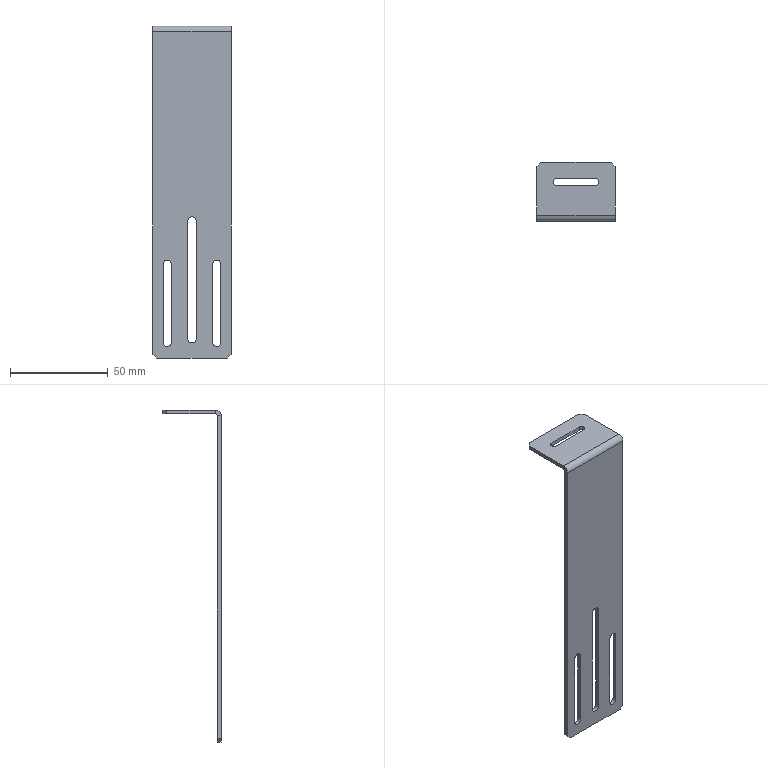Part | NX | 1 solid | 34 faces | box 40 x 30 x 170 mm | volume 14302 mm3 | plane 24 | cylinder 10 | commonest cylinder face diameters 4.2 x4 3.4 x2 4.5 x2 2 x1 6 x1
STEP:
#1=CARTESIAN_POINT('',(14.8,-2.,48.));
#2=VERTEX_POINT('',#1);
#3=CARTESIAN_POINT('',(14.8,-2.,8.));
#4=VERTEX_POINT('',#3);
#5=CARTESIAN_POINT('',(14.8,-2.,8.));
#6=DIRECTION('',(0.,0.,-1.));
#7=VECTOR('',#6,1000.);
#8=LINE('',#5,#7);
#9=EDGE_CURVE('',#2,#4,#8,.T.);
#10=ORIENTED_EDGE('',*,*,#9,.T.);
#11=CARTESIAN_POINT('',(10.6,-2.,8.));
#12=VERTEX_POINT('',#11);
#13=CARTESIAN_POINT('',(12.7,-2.,8.));
#14=DIRECTION('',(0.,1.,0.));
#15=DIRECTION('',(-1.,0.,0.));
#16=AXIS2_PLACEMENT_3D('',#13,#14,#15);
#17=CIRCLE('',#16,2.1);
#18=EDGE_CURVE('',#4,#12,#17,.T.);
#19=ORIENTED_EDGE('',*,*,#18,.T.);
#20=CARTESIAN_POINT('',(10.6,-2.,48.));
#21=VERTEX_POINT('',#20);
#22=CARTESIAN_POINT('',(10.6,-2.,8.));
#23=DIRECTION('',(0.,0.,1.));
#24=VECTOR('',#23,1000.);
#25=LINE('',#22,#24);
#26=EDGE_CURVE('',#12,#21,#25,.T.);
#27=ORIENTED_EDGE('',*,*,#26,.T.);
#28=CARTESIAN_POINT('',(12.7,-2.,48.));
#29=DIRECTION('',(0.,1.,0.));
#30=DIRECTION('',(-1.,0.,0.));
#31=AXIS2_PLACEMENT_3D('',#28,#29,#30);
#32=CIRCLE('',#31,2.1);
#33=EDGE_CURVE('',#21,#2,#32,.T.);
#34=ORIENTED_EDGE('',*,*,#33,.T.);
#35=EDGE_LOOP('',(#10,#19,#27,#34));
#36=FACE_BOUND('',#35,.T.);
#37=CARTESIAN_POINT('',(-10.6,-2.,48.));
#38=VERTEX_POINT('',#37);
#39=CARTESIAN_POINT('',(-10.6,-2.,8.));
#40=VERTEX_POINT('',#39);
#41=CARTESIAN_POINT('',(-10.6,-2.,8.));
#42=DIRECTION('',(0.,0.,-1.));
#43=VECTOR('',#42,1000.);
#44=LINE('',#41,#43);
#45=EDGE_CURVE('',#38,#40,#44,.T.);
#46=ORIENTED_EDGE('',*,*,#45,.T.);
#47=CARTESIAN_POINT('',(-14.8,-2.,8.));
#48=VERTEX_POINT('',#47);
#49=CARTESIAN_POINT('',(-12.7,-2.,8.));
#50=DIRECTION('',(0.,1.,0.));
#51=DIRECTION('',(-1.,0.,0.));
#52=AXIS2_PLACEMENT_3D('',#49,#50,#51);
#53=CIRCLE('',#52,2.1);
#54=EDGE_CURVE('',#40,#48,#53,.T.);
#55=ORIENTED_EDGE('',*,*,#54,.T.);
#56=CARTESIAN_POINT('',(-14.8,-2.,48.));
#57=VERTEX_POINT('',#56);
#58=CARTESIAN_POINT('',(-14.8,-2.,8.));
#59=DIRECTION('',(0.,0.,1.));
#60=VECTOR('',#59,1000.);
#61=LINE('',#58,#60);
#62=EDGE_CURVE('',#48,#57,#61,.T.);
#63=ORIENTED_EDGE('',*,*,#62,.T.);
#64=CARTESIAN_POINT('',(-12.7,-2.,48.));
#65=DIRECTION('',(0.,1.,0.));
#66=DIRECTION('',(-1.,0.,0.));
#67=AXIS2_PLACEMENT_3D('',#64,#65,#66);
#68=CIRCLE('',#67,2.1);
#69=EDGE_CURVE('',#57,#38,#68,.T.);
#70=ORIENTED_EDGE('',*,*,#69,.T.);
#71=EDGE_LOOP('',(#46,#55,#63,#70));
#72=FACE_BOUND('',#71,.T.);
#73=CARTESIAN_POINT('',(2.25,-2.,10.));
#74=VERTEX_POINT('',#73);
#75=CARTESIAN_POINT('',(2.25,-2.,70.));
#76=VERTEX_POINT('',#75);
#77=CARTESIAN_POINT('',(2.25,-2.,10.));
#78=DIRECTION('',(0.,0.,1.));
#79=VECTOR('',#78,1000.);
#80=LINE('',#77,#79);
#81=EDGE_CURVE('',#74,#76,#80,.T.);
#82=ORIENTED_EDGE('',*,*,#81,.F.);
#83=CARTESIAN_POINT('',(-2.25,-2.,10.));
#84=VERTEX_POINT('',#83);
#85=CARTESIAN_POINT('',(0.,-2.,10.));
#86=DIRECTION('',(0.,-1.,0.));
#87=DIRECTION('',(0.,0.,-1.));
#88=AXIS2_PLACEMENT_3D('',#85,#86,#87);
#89=CIRCLE('',#88,2.25);
#90=EDGE_CURVE('',#84,#74,#89,.T.);
#91=ORIENTED_EDGE('',*,*,#90,.F.);
#92=CARTESIAN_POINT('',(-2.25,-2.,70.));
#93=VERTEX_POINT('',#92);
#94=CARTESIAN_POINT('',(-2.25,-2.,10.));
#95=DIRECTION('',(0.,0.,-1.));
#96=VECTOR('',#95,1000.);
#97=LINE('',#94,#96);
#98=EDGE_CURVE('',#93,#84,#97,.T.);
#99=ORIENTED_EDGE('',*,*,#98,.F.);
#100=CARTESIAN_POINT('',(0.,-2.,70.));
#101=DIRECTION('',(0.,-1.,0.));
#102=DIRECTION('',(0.,0.,-1.));
#103=AXIS2_PLACEMENT_3D('',#100,#101,#102);
#104=CIRCLE('',#103,2.25);
#105=EDGE_CURVE('',#76,#93,#104,.T.);
#106=ORIENTED_EDGE('',*,*,#105,.F.);
#107=EDGE_LOOP('',(#82,#91,#99,#106));
#108=FACE_BOUND('',#107,.T.);
#109=CARTESIAN_POINT('',(-20.,-2.,167.));
#110=VERTEX_POINT('',#109);
#111=CARTESIAN_POINT('',(-20.,-2.,2.));
#112=VERTEX_POINT('',#111);
#113=CARTESIAN_POINT('',(-20.,-2.,170.));
#114=DIRECTION('',(0.,0.,-1.));
#115=VECTOR('',#114,1000.);
#116=LINE('',#113,#115);
#117=EDGE_CURVE('',#110,#112,#116,.T.);
#118=ORIENTED_EDGE('',*,*,#117,.T.);
#119=CARTESIAN_POINT('',(-18.,-2.,0.));
#120=VERTEX_POINT('',#119);
#121=CARTESIAN_POINT('',(-18.,-2.,0.));
#122=DIRECTION('',(-0.7071,0.,0.7071));
#123=VECTOR('',#122,1000.);
#124=LINE('',#121,#123);
#125=EDGE_CURVE('',#112,#120,#124,.F.);
#126=ORIENTED_EDGE('',*,*,#125,.T.);
#127=CARTESIAN_POINT('',(18.,-2.,0.));
#128=VERTEX_POINT('',#127);
#129=CARTESIAN_POINT('',(-20.,-2.,0.));
#130=DIRECTION('',(1.,0.,0.));
#131=VECTOR('',#130,1000.);
#132=LINE('',#129,#131);
#133=EDGE_CURVE('',#120,#128,#132,.T.);
#134=ORIENTED_EDGE('',*,*,#133,.T.);
#135=CARTESIAN_POINT('',(20.,-2.,2.));
#136=VERTEX_POINT('',#135);
#137=CARTESIAN_POINT('',(18.,-2.,0.));
#138=DIRECTION('',(-0.7071,0.,-0.7071));
#139=VECTOR('',#138,1000.);
#140=LINE('',#137,#139);
#141=EDGE_CURVE('',#128,#136,#140,.F.);
#142=ORIENTED_EDGE('',*,*,#141,.T.);
#143=CARTESIAN_POINT('',(20.,-2.,167.));
#144=VERTEX_POINT('',#143);
#145=CARTESIAN_POINT('',(20.,-2.,170.));
#146=DIRECTION('',(0.,0.,-1.));
#147=VECTOR('',#146,1000.);
#148=LINE('',#145,#147);
#149=EDGE_CURVE('',#144,#136,#148,.T.);
#150=ORIENTED_EDGE('',*,*,#149,.F.);
#151=CARTESIAN_POINT('',(20.,-2.,167.));
#152=DIRECTION('',(1.,0.,0.));
#153=VECTOR('',#152,1000.);
#154=LINE('',#151,#153);
#155=EDGE_CURVE('',#144,#110,#154,.F.);
#156=ORIENTED_EDGE('',*,*,#155,.T.);
#157=EDGE_LOOP('',(#118,#126,#134,#142,#150,#156));
#158=FACE_BOUND('',#157,.T.);
#159=CARTESIAN_POINT('',(-20.,-2.,170.));
#160=DIRECTION('',(0.,1.,0.));
#161=DIRECTION('',(0.,0.,1.));
#162=AXIS2_PLACEMENT_3D('',#159,#160,#161);
#163=PLANE('',#162);
#164=ADVANCED_FACE('',(#36,#72,#108,#158),#163,.F.);
#165=ORIENTED_EDGE('',*,*,#149,.T.);
#166=CARTESIAN_POINT('',(20.,0.,2.));
#167=VERTEX_POINT('',#166);
#168=CARTESIAN_POINT('',(20.,0.,2.));
#169=DIRECTION('',(0.,1.,0.));
#170=VECTOR('',#169,1000.);
#171=LINE('',#168,#170);
#172=EDGE_CURVE('',#136,#167,#171,.T.);
#173=ORIENTED_EDGE('',*,*,#172,.T.);
#174=CARTESIAN_POINT('',(20.,0.,167.));
#175=VERTEX_POINT('',#174);
#176=CARTESIAN_POINT('',(20.,0.,170.));
#177=DIRECTION('',(0.,0.,-1.));
#178=VECTOR('',#177,1000.);
#179=LINE('',#176,#178);
#180=EDGE_CURVE('',#175,#167,#179,.T.);
#181=ORIENTED_EDGE('',*,*,#180,.F.);
#182=CARTESIAN_POINT('',(20.,0.,167.));
#183=DIRECTION('',(0.,-1.,0.));
#184=VECTOR('',#183,1000.);
#185=LINE('',#182,#184);
#186=EDGE_CURVE('',#175,#144,#185,.T.);
#187=ORIENTED_EDGE('',*,*,#186,.T.);
#188=EDGE_LOOP('',(#165,#173,#181,#187));
#189=FACE_BOUND('',#188,.T.);
#190=CARTESIAN_POINT('',(20.,0.,170.));
#191=DIRECTION('',(1.,0.,0.));
#192=DIRECTION('',(0.,0.,-1.));
#193=AXIS2_PLACEMENT_3D('',#190,#191,#192);
#194=PLANE('',#193);
#195=ADVANCED_FACE('',(#189),#194,.T.);
#196=CARTESIAN_POINT('',(14.8,0.,8.));
#197=VERTEX_POINT('',#196);
#198=CARTESIAN_POINT('',(10.6,0.,8.));
#199=VERTEX_POINT('',#198);
#200=CARTESIAN_POINT('',(12.7,0.,8.));
#201=DIRECTION('',(0.,1.,0.));
#202=DIRECTION('',(-1.,0.,0.));
#203=AXIS2_PLACEMENT_3D('',#200,#201,#202);
#204=CIRCLE('',#203,2.1);
#205=EDGE_CURVE('',#197,#199,#204,.T.);
#206=ORIENTED_EDGE('',*,*,#205,.F.);
#207=CARTESIAN_POINT('',(14.8,0.,48.));
#208=VERTEX_POINT('',#207);
#209=CARTESIAN_POINT('',(14.8,0.,8.));
#210=DIRECTION('',(0.,0.,-1.));
#211=VECTOR('',#210,1000.);
#212=LINE('',#209,#211);
#213=EDGE_CURVE('',#208,#197,#212,.T.);
#214=ORIENTED_EDGE('',*,*,#213,.F.);
#215=CARTESIAN_POINT('',(10.6,0.,48.));
#216=VERTEX_POINT('',#215);
#217=CARTESIAN_POINT('',(12.7,0.,48.));
#218=DIRECTION('',(0.,1.,0.));
#219=DIRECTION('',(-1.,0.,0.));
#220=AXIS2_PLACEMENT_3D('',#217,#218,#219);
#221=CIRCLE('',#220,2.1);
#222=EDGE_CURVE('',#216,#208,#221,.T.);
#223=ORIENTED_EDGE('',*,*,#222,.F.);
#224=CARTESIAN_POINT('',(10.6,0.,8.));
#225=DIRECTION('',(0.,0.,1.));
#226=VECTOR('',#225,1000.);
#227=LINE('',#224,#226);
#228=EDGE_CURVE('',#199,#216,#227,.T.);
#229=ORIENTED_EDGE('',*,*,#228,.F.);
#230=EDGE_LOOP('',(#206,#214,#223,#229));
#231=FACE_BOUND('',#230,.T.);
#232=CARTESIAN_POINT('',(-10.6,0.,8.));
#233=VERTEX_POINT('',#232);
#234=CARTESIAN_POINT('',(-14.8,0.,8.));
#235=VERTEX_POINT('',#234);
#236=CARTESIAN_POINT('',(-12.7,0.,8.));
#237=DIRECTION('',(0.,1.,0.));
#238=DIRECTION('',(-1.,0.,0.));
#239=AXIS2_PLACEMENT_3D('',#236,#237,#238);
#240=CIRCLE('',#239,2.1);
#241=EDGE_CURVE('',#233,#235,#240,.T.);
#242=ORIENTED_EDGE('',*,*,#241,.F.);
#243=CARTESIAN_POINT('',(-10.6,0.,48.));
#244=VERTEX_POINT('',#243);
#245=CARTESIAN_POINT('',(-10.6,0.,8.));
#246=DIRECTION('',(0.,0.,-1.));
#247=VECTOR('',#246,1000.);
#248=LINE('',#245,#247);
#249=EDGE_CURVE('',#244,#233,#248,.T.);
#250=ORIENTED_EDGE('',*,*,#249,.F.);
#251=CARTESIAN_POINT('',(-14.8,0.,48.));
#252=VERTEX_POINT('',#251);
#253=CARTESIAN_POINT('',(-12.7,0.,48.));
#254=DIRECTION('',(0.,1.,0.));
#255=DIRECTION('',(-1.,0.,0.));
#256=AXIS2_PLACEMENT_3D('',#253,#254,#255);
#257=CIRCLE('',#256,2.1);
#258=EDGE_CURVE('',#252,#244,#257,.T.);
#259=ORIENTED_EDGE('',*,*,#258,.F.);
#260=CARTESIAN_POINT('',(-14.8,0.,8.));
#261=DIRECTION('',(0.,0.,1.));
#262=VECTOR('',#261,1000.);
#263=LINE('',#260,#262);
#264=EDGE_CURVE('',#235,#252,#263,.T.);
#265=ORIENTED_EDGE('',*,*,#264,.F.);
#266=EDGE_LOOP('',(#242,#250,#259,#265));
#267=FACE_BOUND('',#266,.T.);
#268=CARTESIAN_POINT('',(-2.25,0.,10.));
#269=VERTEX_POINT('',#268);
#270=CARTESIAN_POINT('',(2.25,0.,10.));
#271=VERTEX_POINT('',#270);
#272=CARTESIAN_POINT('',(0.,0.,10.));
#273=DIRECTION('',(0.,-1.,0.));
#274=DIRECTION('',(0.,0.,-1.));
#275=AXIS2_PLACEMENT_3D('',#272,#273,#274);
#276=CIRCLE('',#275,2.25);
#277=EDGE_CURVE('',#269,#271,#276,.T.);
#278=ORIENTED_EDGE('',*,*,#277,.T.);
#279=CARTESIAN_POINT('',(2.25,0.,70.));
#280=VERTEX_POINT('',#279);
#281=CARTESIAN_POINT('',(2.25,0.,10.));
#282=DIRECTION('',(0.,0.,1.));
#283=VECTOR('',#282,1000.);
#284=LINE('',#281,#283);
#285=EDGE_CURVE('',#271,#280,#284,.T.);
#286=ORIENTED_EDGE('',*,*,#285,.T.);
#287=CARTESIAN_POINT('',(-2.25,0.,70.));
#288=VERTEX_POINT('',#287);
#289=CARTESIAN_POINT('',(0.,0.,70.));
#290=DIRECTION('',(0.,-1.,0.));
#291=DIRECTION('',(0.,0.,-1.));
#292=AXIS2_PLACEMENT_3D('',#289,#290,#291);
#293=CIRCLE('',#292,2.25);
#294=EDGE_CURVE('',#280,#288,#293,.T.);
#295=ORIENTED_EDGE('',*,*,#294,.T.);
#296=CARTESIAN_POINT('',(-2.25,0.,10.));
#297=DIRECTION('',(0.,0.,-1.));
#298=VECTOR('',#297,1000.);
#299=LINE('',#296,#298);
#300=EDGE_CURVE('',#288,#269,#299,.T.);
#301=ORIENTED_EDGE('',*,*,#300,.T.);
#302=EDGE_LOOP('',(#278,#286,#295,#301));
#303=FACE_BOUND('',#302,.T.);
#304=CARTESIAN_POINT('',(-18.,0.,0.));
#305=VERTEX_POINT('',#304);
#306=CARTESIAN_POINT('',(18.,0.,0.));
#307=VERTEX_POINT('',#306);
#308=CARTESIAN_POINT('',(-20.,0.,0.));
#309=DIRECTION('',(1.,0.,0.));
#310=VECTOR('',#309,1000.);
#311=LINE('',#308,#310);
#312=EDGE_CURVE('',#305,#307,#311,.T.);
#313=ORIENTED_EDGE('',*,*,#312,.F.);
#314=CARTESIAN_POINT('',(-20.,0.,2.));
#315=VERTEX_POINT('',#314);
#316=CARTESIAN_POINT('',(-104.,0.,86.));
#317=DIRECTION('',(0.7071,0.,-0.7071));
#318=VECTOR('',#317,1000.);
#319=LINE('',#316,#318);
#320=EDGE_CURVE('',#305,#315,#319,.F.);
#321=ORIENTED_EDGE('',*,*,#320,.T.);
#322=CARTESIAN_POINT('',(-20.,0.,167.));
#323=VERTEX_POINT('',#322);
#324=CARTESIAN_POINT('',(-20.,0.,170.));
#325=DIRECTION('',(0.,0.,-1.));
#326=VECTOR('',#325,1000.);
#327=LINE('',#324,#326);
#328=EDGE_CURVE('',#323,#315,#327,.T.);
#329=ORIENTED_EDGE('',*,*,#328,.F.);
#330=CARTESIAN_POINT('',(20.,0.,167.));
#331=DIRECTION('',(1.,0.,0.));
#332=VECTOR('',#331,1000.);
#333=LINE('',#330,#332);
#334=EDGE_CURVE('',#175,#323,#333,.F.);
#335=ORIENTED_EDGE('',*,*,#334,.F.);
#336=ORIENTED_EDGE('',*,*,#180,.T.);
#337=CARTESIAN_POINT('',(84.,0.,66.));
#338=DIRECTION('',(0.7071,0.,0.7071));
#339=VECTOR('',#338,1000.);
#340=LINE('',#337,#339);
#341=EDGE_CURVE('',#167,#307,#340,.F.);
#342=ORIENTED_EDGE('',*,*,#341,.T.);
#343=EDGE_LOOP('',(#313,#321,#329,#335,#336,#342));
#344=FACE_BOUND('',#343,.T.);
#345=CARTESIAN_POINT('',(-20.,0.,170.));
#346=DIRECTION('',(0.,1.,0.));
#347=DIRECTION('',(0.,0.,1.));
#348=AXIS2_PLACEMENT_3D('',#345,#346,#347);
#349=PLANE('',#348);
#350=ADVANCED_FACE('',(#231,#267,#303,#344),#349,.T.);
#351=ORIENTED_EDGE('',*,*,#328,.T.);
#352=CARTESIAN_POINT('',(-20.,-2.,2.));
#353=DIRECTION('',(0.,-1.,0.));
#354=VECTOR('',#353,1000.);
#355=LINE('',#352,#354);
#356=EDGE_CURVE('',#315,#112,#355,.T.);
#357=ORIENTED_EDGE('',*,*,#356,.T.);
#358=ORIENTED_EDGE('',*,*,#117,.F.);
#359=CARTESIAN_POINT('',(-20.,0.,167.));
#360=DIRECTION('',(0.,-1.,0.));
#361=VECTOR('',#360,1000.);
#362=LINE('',#359,#361);
#363=EDGE_CURVE('',#323,#110,#362,.T.);
#364=ORIENTED_EDGE('',*,*,#363,.F.);
#365=EDGE_LOOP('',(#351,#357,#358,#364));
#366=FACE_BOUND('',#365,.T.);
#367=CARTESIAN_POINT('',(-20.,-2.,170.));
#368=DIRECTION('',(-1.,0.,0.));
#369=DIRECTION('',(0.,0.,1.));
#370=AXIS2_PLACEMENT_3D('',#367,#368,#369);
#371=PLANE('',#370);
#372=ADVANCED_FACE('',(#366),#371,.T.);
#373=ORIENTED_EDGE('',*,*,#133,.F.);
#374=CARTESIAN_POINT('',(-18.,0.,0.));
#375=DIRECTION('',(0.,1.,0.));
#376=VECTOR('',#375,1000.);
#377=LINE('',#374,#376);
#378=EDGE_CURVE('',#120,#305,#377,.T.);
#379=ORIENTED_EDGE('',*,*,#378,.T.);
#380=ORIENTED_EDGE('',*,*,#312,.T.);
#381=CARTESIAN_POINT('',(18.,0.,0.));
#382=DIRECTION('',(0.,-1.,0.));
#383=VECTOR('',#382,1000.);
#384=LINE('',#381,#383);
#385=EDGE_CURVE('',#307,#128,#384,.T.);
#386=ORIENTED_EDGE('',*,*,#385,.T.);
#387=EDGE_LOOP('',(#373,#379,#380,#386));
#388=FACE_BOUND('',#387,.T.);
#389=CARTESIAN_POINT('',(0.,0.,0.));
#390=DIRECTION('',(0.,0.,-1.));
#391=DIRECTION('',(-1.,0.,0.));
#392=AXIS2_PLACEMENT_3D('',#389,#390,#391);
#393=PLANE('',#392);
#394=ADVANCED_FACE('',(#388),#393,.T.);
#395=CARTESIAN_POINT('',(-20.,1.,168.));
#396=VERTEX_POINT('',#395);
#397=CARTESIAN_POINT('',(-20.,1.,170.));
#398=VERTEX_POINT('',#397);
#399=CARTESIAN_POINT('',(-20.,1.,170.));
#400=DIRECTION('',(0.,0.,-1.));
#401=VECTOR('',#400,1000.);
#402=LINE('',#399,#401);
#403=EDGE_CURVE('',#396,#398,#402,.F.);
#404=ORIENTED_EDGE('',*,*,#403,.F.);
#405=CARTESIAN_POINT('',(-20.,1.,167.));
#406=DIRECTION('',(1.,0.,0.));
#407=DIRECTION('',(0.,0.,-1.));
#408=AXIS2_PLACEMENT_3D('',#405,#406,#407);
#409=CIRCLE('',#408,1.);
#410=EDGE_CURVE('',#323,#396,#409,.F.);
#411=ORIENTED_EDGE('',*,*,#410,.F.);
#412=ORIENTED_EDGE('',*,*,#363,.T.);
#413=CARTESIAN_POINT('',(-20.,1.,167.));
#414=DIRECTION('',(1.,0.,0.));
#415=DIRECTION('',(0.,0.,-1.));
#416=AXIS2_PLACEMENT_3D('',#413,#414,#415);
#417=CIRCLE('',#416,3.);
#418=EDGE_CURVE('',#110,#398,#417,.F.);
#419=ORIENTED_EDGE('',*,*,#418,.T.);
#420=EDGE_LOOP('',(#404,#411,#412,#419));
#421=FACE_BOUND('',#420,.T.);
#422=CARTESIAN_POINT('',(-20.,1.,167.));
#423=DIRECTION('',(-1.,0.,0.));
#424=DIRECTION('',(0.,0.,1.));
#425=AXIS2_PLACEMENT_3D('',#422,#423,#424);
#426=PLANE('',#425);
#427=ADVANCED_FACE('',(#421),#426,.T.);
#428=CARTESIAN_POINT('',(20.,1.,168.));
#429=VERTEX_POINT('',#428);
#430=CARTESIAN_POINT('',(20.,1.,167.));
#431=DIRECTION('',(1.,0.,0.));
#432=DIRECTION('',(0.,0.,-1.));
#433=AXIS2_PLACEMENT_3D('',#430,#431,#432);
#434=CIRCLE('',#433,1.);
#435=EDGE_CURVE('',#429,#175,#434,.T.);
#436=ORIENTED_EDGE('',*,*,#435,.F.);
#437=CARTESIAN_POINT('',(20.,1.,170.));
#438=VERTEX_POINT('',#437);
#439=CARTESIAN_POINT('',(20.,1.,168.));
#440=DIRECTION('',(0.,0.,-1.));
#441=VECTOR('',#440,1000.);
#442=LINE('',#439,#441);
#443=EDGE_CURVE('',#429,#438,#442,.F.);
#444=ORIENTED_EDGE('',*,*,#443,.T.);
#445=CARTESIAN_POINT('',(20.,1.,167.));
#446=DIRECTION('',(1.,0.,0.));
#447=DIRECTION('',(0.,0.,-1.));
#448=AXIS2_PLACEMENT_3D('',#445,#446,#447);
#449=CIRCLE('',#448,3.);
#450=EDGE_CURVE('',#438,#144,#449,.T.);
#451=ORIENTED_EDGE('',*,*,#450,.T.);
#452=ORIENTED_EDGE('',*,*,#186,.F.);
#453=EDGE_LOOP('',(#436,#444,#451,#452));
#454=FACE_BOUND('',#453,.T.);
#455=CARTESIAN_POINT('',(20.,1.,167.));
#456=DIRECTION('',(-1.,0.,0.));
#457=DIRECTION('',(0.,0.,1.));
#458=AXIS2_PLACEMENT_3D('',#455,#456,#457);
#459=PLANE('',#458);
#460=ADVANCED_FACE('',(#454),#459,.F.);
#461=ORIENTED_EDGE('',*,*,#155,.F.);
#462=ORIENTED_EDGE('',*,*,#450,.F.);
#463=CARTESIAN_POINT('',(-20.,1.,170.));
#464=DIRECTION('',(1.,0.,0.));
#465=VECTOR('',#464,1000.);
#466=LINE('',#463,#465);
#467=EDGE_CURVE('',#438,#398,#466,.F.);
#468=ORIENTED_EDGE('',*,*,#467,.T.);
#469=ORIENTED_EDGE('',*,*,#418,.F.);
#470=EDGE_LOOP('',(#461,#462,#468,#469));
#471=FACE_BOUND('',#470,.T.);
#472=CARTESIAN_POINT('',(20.,1.,167.));
#473=DIRECTION('',(1.,0.,0.));
#474=DIRECTION('',(0.,0.,1.));
#475=AXIS2_PLACEMENT_3D('',#472,#473,#474);
#476=CYLINDRICAL_SURFACE('',#475,3.);
#477=ADVANCED_FACE('',(#471),#476,.T.);
#478=ORIENTED_EDGE('',*,*,#334,.T.);
#479=ORIENTED_EDGE('',*,*,#410,.T.);
#480=CARTESIAN_POINT('',(-20.,1.,168.));
#481=DIRECTION('',(1.,0.,0.));
#482=VECTOR('',#481,1000.);
#483=LINE('',#480,#482);
#484=EDGE_CURVE('',#396,#429,#483,.T.);
#485=ORIENTED_EDGE('',*,*,#484,.T.);
#486=ORIENTED_EDGE('',*,*,#435,.T.);
#487=EDGE_LOOP('',(#478,#479,#485,#486));
#488=FACE_BOUND('',#487,.T.);
#489=CARTESIAN_POINT('',(20.,1.,167.));
#490=DIRECTION('',(1.,0.,0.));
#491=DIRECTION('',(0.,0.,1.));
#492=AXIS2_PLACEMENT_3D('',#489,#490,#491);
#493=CYLINDRICAL_SURFACE('',#492,1.);
#494=ADVANCED_FACE('',(#488),#493,.F.);
#495=CARTESIAN_POINT('',(-20.,26.,170.));
#496=VERTEX_POINT('',#495);
#497=CARTESIAN_POINT('',(-20.,0.,170.));
#498=DIRECTION('',(0.,-1.,0.));
#499=VECTOR('',#498,1000.);
#500=LINE('',#497,#499);
#501=EDGE_CURVE('',#496,#398,#500,.T.);
#502=ORIENTED_EDGE('',*,*,#501,.F.);
#503=CARTESIAN_POINT('',(-20.,26.,168.));
#504=VERTEX_POINT('',#503);
#505=CARTESIAN_POINT('',(-20.,26.,170.));
#506=DIRECTION('',(0.,0.,-1.));
#507=VECTOR('',#506,1000.);
#508=LINE('',#505,#507);
#509=EDGE_CURVE('',#496,#504,#508,.T.);
#510=ORIENTED_EDGE('',*,*,#509,.T.);
#511=CARTESIAN_POINT('',(-20.,0.,168.));
#512=DIRECTION('',(0.,1.,0.));
#513=VECTOR('',#512,1000.);
#514=LINE('',#511,#513);
#515=EDGE_CURVE('',#504,#396,#514,.F.);
#516=ORIENTED_EDGE('',*,*,#515,.T.);
#517=ORIENTED_EDGE('',*,*,#403,.T.);
#518=EDGE_LOOP('',(#502,#510,#516,#517));
#519=FACE_BOUND('',#518,.T.);
#520=CARTESIAN_POINT('',(-20.,0.,170.));
#521=DIRECTION('',(1.,0.,0.));
#522=DIRECTION('',(0.,0.,-1.));
#523=AXIS2_PLACEMENT_3D('',#520,#521,#522);
#524=PLANE('',#523);
#525=ADVANCED_FACE('',(#519),#524,.F.);
#526=CARTESIAN_POINT('',(20.,26.,168.));
#527=VERTEX_POINT('',#526);
#528=CARTESIAN_POINT('',(20.,28.,168.));
#529=DIRECTION('',(0.,-1.,0.));
#530=VECTOR('',#529,1000.);
#531=LINE('',#528,#530);
#532=EDGE_CURVE('',#429,#527,#531,.F.);
#533=ORIENTED_EDGE('',*,*,#532,.T.);
#534=CARTESIAN_POINT('',(20.,26.,170.));
#535=VERTEX_POINT('',#534);
#536=CARTESIAN_POINT('',(20.,26.,170.));
#537=DIRECTION('',(0.,0.,1.));
#538=VECTOR('',#537,1000.);
#539=LINE('',#536,#538);
#540=EDGE_CURVE('',#527,#535,#539,.T.);
#541=ORIENTED_EDGE('',*,*,#540,.T.);
#542=CARTESIAN_POINT('',(20.,0.,170.));
#543=DIRECTION('',(0.,1.,0.));
#544=VECTOR('',#543,1000.);
#545=LINE('',#542,#544);
#546=EDGE_CURVE('',#438,#535,#545,.T.);
#547=ORIENTED_EDGE('',*,*,#546,.F.);
#548=ORIENTED_EDGE('',*,*,#443,.F.);
#549=EDGE_LOOP('',(#533,#541,#547,#548));
#550=FACE_BOUND('',#549,.T.);
#551=CARTESIAN_POINT('',(20.,28.,170.));
#552=DIRECTION('',(-1.,0.,0.));
#553=DIRECTION('',(0.,-1.,0.));
#554=AXIS2_PLACEMENT_3D('',#551,#552,#553);
#555=PLANE('',#554);
#556=ADVANCED_FACE('',(#550),#555,.F.);
#557=CARTESIAN_POINT('',(-10.,16.3,170.));
#558=VERTEX_POINT('',#557);
#559=CARTESIAN_POINT('',(10.,16.3,170.));
#560=VERTEX_POINT('',#559);
#561=CARTESIAN_POINT('',(-10.,16.3,170.));
#562=DIRECTION('',(1.,0.,0.));
#563=VECTOR('',#562,1000.);
#564=LINE('',#561,#563);
#565=EDGE_CURVE('',#558,#560,#564,.T.);
#566=ORIENTED_EDGE('',*,*,#565,.F.);
#567=CARTESIAN_POINT('',(-10.,19.7,170.));
#568=VERTEX_POINT('',#567);
#569=CARTESIAN_POINT('',(-10.,18.,170.));
#570=DIRECTION('',(0.,0.,1.));
#571=DIRECTION('',(1.,0.,0.));
#572=AXIS2_PLACEMENT_3D('',#569,#570,#571);
#573=CIRCLE('',#572,1.7);
#574=EDGE_CURVE('',#568,#558,#573,.T.);
#575=ORIENTED_EDGE('',*,*,#574,.F.);
#576=CARTESIAN_POINT('',(10.,19.7,170.));
#577=VERTEX_POINT('',#576);
#578=CARTESIAN_POINT('',(-10.,19.7,170.));
#579=DIRECTION('',(-1.,0.,0.));
#580=VECTOR('',#579,1000.);
#581=LINE('',#578,#580);
#582=EDGE_CURVE('',#577,#568,#581,.T.);
#583=ORIENTED_EDGE('',*,*,#582,.F.);
#584=CARTESIAN_POINT('',(10.,18.,170.));
#585=DIRECTION('',(0.,0.,1.));
#586=DIRECTION('',(1.,0.,0.));
#587=AXIS2_PLACEMENT_3D('',#584,#585,#586);
#588=CIRCLE('',#587,1.7);
#589=EDGE_CURVE('',#560,#577,#588,.T.);
#590=ORIENTED_EDGE('',*,*,#589,.F.);
#591=EDGE_LOOP('',(#566,#575,#583,#590));
#592=FACE_BOUND('',#591,.T.);
#593=ORIENTED_EDGE('',*,*,#546,.T.);
#594=CARTESIAN_POINT('',(18.,28.,170.));
#595=VERTEX_POINT('',#594);
#596=CARTESIAN_POINT('',(18.,28.,170.));
#597=DIRECTION('',(0.7071,-0.7071,0.));
#598=VECTOR('',#597,1000.);
#599=LINE('',#596,#598);
#600=EDGE_CURVE('',#535,#595,#599,.F.);
#601=ORIENTED_EDGE('',*,*,#600,.T.);
#602=CARTESIAN_POINT('',(-18.,28.,170.));
#603=VERTEX_POINT('',#602);
#604=CARTESIAN_POINT('',(0.,28.,170.));
#605=DIRECTION('',(-1.,0.,0.));
#606=VECTOR('',#605,1000.);
#607=LINE('',#604,#606);
#608=EDGE_CURVE('',#595,#603,#607,.T.);
#609=ORIENTED_EDGE('',*,*,#608,.T.);
#610=CARTESIAN_POINT('',(-20.,26.,170.));
#611=DIRECTION('',(0.7071,0.7071,0.));
#612=VECTOR('',#611,1000.);
#613=LINE('',#610,#612);
#614=EDGE_CURVE('',#603,#496,#613,.F.);
#615=ORIENTED_EDGE('',*,*,#614,.T.);
#616=ORIENTED_EDGE('',*,*,#501,.T.);
#617=ORIENTED_EDGE('',*,*,#467,.F.);
#618=EDGE_LOOP('',(#593,#601,#609,#615,#616,#617));
#619=FACE_BOUND('',#618,.T.);
#620=CARTESIAN_POINT('',(0.,0.,170.));
#621=DIRECTION('',(0.,0.,-1.));
#622=DIRECTION('',(-1.,0.,0.));
#623=AXIS2_PLACEMENT_3D('',#620,#621,#622);
#624=PLANE('',#623);
#625=ADVANCED_FACE('',(#592,#619),#624,.F.);
#626=CARTESIAN_POINT('',(-10.,19.7,168.));
#627=VERTEX_POINT('',#626);
#628=CARTESIAN_POINT('',(-10.,16.3,168.));
#629=VERTEX_POINT('',#628);
#630=CARTESIAN_POINT('',(-10.,18.,168.));
#631=DIRECTION('',(0.,0.,1.));
#632=DIRECTION('',(1.,0.,0.));
#633=AXIS2_PLACEMENT_3D('',#630,#631,#632);
#634=CIRCLE('',#633,1.7);
#635=EDGE_CURVE('',#627,#629,#634,.T.);
#636=ORIENTED_EDGE('',*,*,#635,.T.);
#637=CARTESIAN_POINT('',(10.,16.3,168.));
#638=VERTEX_POINT('',#637);
#639=CARTESIAN_POINT('',(-10.,16.3,168.));
#640=DIRECTION('',(1.,0.,0.));
#641=VECTOR('',#640,1000.);
#642=LINE('',#639,#641);
#643=EDGE_CURVE('',#629,#638,#642,.T.);
#644=ORIENTED_EDGE('',*,*,#643,.T.);
#645=CARTESIAN_POINT('',(10.,19.7,168.));
#646=VERTEX_POINT('',#645);
#647=CARTESIAN_POINT('',(10.,18.,168.));
#648=DIRECTION('',(0.,0.,1.));
#649=DIRECTION('',(1.,0.,0.));
#650=AXIS2_PLACEMENT_3D('',#647,#648,#649);
#651=CIRCLE('',#650,1.7);
#652=EDGE_CURVE('',#638,#646,#651,.T.);
#653=ORIENTED_EDGE('',*,*,#652,.T.);
#654=CARTESIAN_POINT('',(-10.,19.7,168.));
#655=DIRECTION('',(-1.,0.,0.));
#656=VECTOR('',#655,1000.);
#657=LINE('',#654,#656);
#658=EDGE_CURVE('',#646,#627,#657,.T.);
#659=ORIENTED_EDGE('',*,*,#658,.T.);
#660=EDGE_LOOP('',(#636,#644,#653,#659));
#661=FACE_BOUND('',#660,.T.);
#662=CARTESIAN_POINT('',(18.,28.,168.));
#663=VERTEX_POINT('',#662);
#664=CARTESIAN_POINT('',(-18.,28.,168.));
#665=VERTEX_POINT('',#664);
#666=CARTESIAN_POINT('',(-20.,28.,168.));
#667=DIRECTION('',(1.,0.,0.));
#668=VECTOR('',#667,1000.);
#669=LINE('',#666,#668);
#670=EDGE_CURVE('',#663,#665,#669,.F.);
#671=ORIENTED_EDGE('',*,*,#670,.F.);
#672=CARTESIAN_POINT('',(23.,23.,168.));
#673=DIRECTION('',(-0.7071,0.7071,0.));
#674=VECTOR('',#673,1000.);
#675=LINE('',#672,#674);
#676=EDGE_CURVE('',#663,#527,#675,.F.);
#677=ORIENTED_EDGE('',*,*,#676,.T.);
#678=ORIENTED_EDGE('',*,*,#532,.F.);
#679=ORIENTED_EDGE('',*,*,#484,.F.);
#680=ORIENTED_EDGE('',*,*,#515,.F.);
#681=CARTESIAN_POINT('',(-23.,23.,168.));
#682=DIRECTION('',(-0.7071,-0.7071,0.));
#683=VECTOR('',#682,1000.);
#684=LINE('',#681,#683);
#685=EDGE_CURVE('',#504,#665,#684,.F.);
#686=ORIENTED_EDGE('',*,*,#685,.T.);
#687=EDGE_LOOP('',(#671,#677,#678,#679,#680,#686));
#688=FACE_BOUND('',#687,.T.);
#689=CARTESIAN_POINT('',(0.,0.,168.));
#690=DIRECTION('',(0.,0.,-1.));
#691=DIRECTION('',(-1.,0.,0.));
#692=AXIS2_PLACEMENT_3D('',#689,#690,#691);
#693=PLANE('',#692);
#694=ADVANCED_FACE('',(#661,#688),#693,.T.);
#695=ORIENTED_EDGE('',*,*,#608,.F.);
#696=CARTESIAN_POINT('',(18.,28.,170.));
#697=DIRECTION('',(0.,0.,-1.));
#698=VECTOR('',#697,1000.);
#699=LINE('',#696,#698);
#700=EDGE_CURVE('',#595,#663,#699,.T.);
#701=ORIENTED_EDGE('',*,*,#700,.T.);
#702=ORIENTED_EDGE('',*,*,#670,.T.);
#703=CARTESIAN_POINT('',(-18.,28.,170.));
#704=DIRECTION('',(0.,0.,1.));
#705=VECTOR('',#704,1000.);
#706=LINE('',#703,#705);
#707=EDGE_CURVE('',#665,#603,#706,.T.);
#708=ORIENTED_EDGE('',*,*,#707,.T.);
#709=EDGE_LOOP('',(#695,#701,#702,#708));
#710=FACE_BOUND('',#709,.T.);
#711=CARTESIAN_POINT('',(-20.,28.,170.));
#712=DIRECTION('',(0.,-1.,0.));
#713=DIRECTION('',(0.,0.,-1.));
#714=AXIS2_PLACEMENT_3D('',#711,#712,#713);
#715=PLANE('',#714);
#716=ADVANCED_FACE('',(#710),#715,.F.);
#717=ORIENTED_EDGE('',*,*,#90,.T.);
#718=CARTESIAN_POINT('',(2.25,0.,10.));
#719=DIRECTION('',(0.,-1.,0.));
#720=VECTOR('',#719,1000.);
#721=LINE('',#718,#720);
#722=EDGE_CURVE('',#271,#74,#721,.T.);
#723=ORIENTED_EDGE('',*,*,#722,.F.);
#724=ORIENTED_EDGE('',*,*,#277,.F.);
#725=CARTESIAN_POINT('',(-2.25,0.,10.));
#726=DIRECTION('',(0.,-1.,0.));
#727=VECTOR('',#726,1000.);
#728=LINE('',#725,#727);
#729=EDGE_CURVE('',#269,#84,#728,.T.);
#730=ORIENTED_EDGE('',*,*,#729,.T.);
#731=EDGE_LOOP('',(#717,#723,#724,#730));
#732=FACE_BOUND('',#731,.T.);
#733=CARTESIAN_POINT('',(0.,0.,10.));
#734=DIRECTION('',(0.,-1.,0.));
#735=DIRECTION('',(0.,0.,-1.));
#736=AXIS2_PLACEMENT_3D('',#733,#734,#735);
#737=CYLINDRICAL_SURFACE('',#736,2.25);
#738=ADVANCED_FACE('',(#732),#737,.F.);
#739=ORIENTED_EDGE('',*,*,#98,.T.);
#740=ORIENTED_EDGE('',*,*,#729,.F.);
#741=ORIENTED_EDGE('',*,*,#300,.F.);
#742=CARTESIAN_POINT('',(-2.25,0.,70.));
#743=DIRECTION('',(0.,-1.,0.));
#744=VECTOR('',#743,1000.);
#745=LINE('',#742,#744);
#746=EDGE_CURVE('',#288,#93,#745,.T.);
#747=ORIENTED_EDGE('',*,*,#746,.T.);
#748=EDGE_LOOP('',(#739,#740,#741,#747));
#749=FACE_BOUND('',#748,.T.);
#750=CARTESIAN_POINT('',(-2.25,0.,10.));
#751=DIRECTION('',(-1.,0.,0.));
#752=DIRECTION('',(0.,0.,1.));
#753=AXIS2_PLACEMENT_3D('',#750,#751,#752);
#754=PLANE('',#753);
#755=ADVANCED_FACE('',(#749),#754,.F.);
#756=ORIENTED_EDGE('',*,*,#105,.T.);
#757=ORIENTED_EDGE('',*,*,#746,.F.);
#758=ORIENTED_EDGE('',*,*,#294,.F.);
#759=CARTESIAN_POINT('',(2.25,0.,70.));
#760=DIRECTION('',(0.,-1.,0.));
#761=VECTOR('',#760,1000.);
#762=LINE('',#759,#761);
#763=EDGE_CURVE('',#280,#76,#762,.T.);
#764=ORIENTED_EDGE('',*,*,#763,.T.);
#765=EDGE_LOOP('',(#756,#757,#758,#764));
#766=FACE_BOUND('',#765,.T.);
#767=CARTESIAN_POINT('',(0.,0.,70.));
#768=DIRECTION('',(0.,-1.,0.));
#769=DIRECTION('',(0.,0.,-1.));
#770=AXIS2_PLACEMENT_3D('',#767,#768,#769);
#771=CYLINDRICAL_SURFACE('',#770,2.25);
#772=ADVANCED_FACE('',(#766),#771,.F.);
#773=ORIENTED_EDGE('',*,*,#81,.T.);
#774=ORIENTED_EDGE('',*,*,#763,.F.);
#775=ORIENTED_EDGE('',*,*,#285,.F.);
#776=ORIENTED_EDGE('',*,*,#722,.T.);
#777=EDGE_LOOP('',(#773,#774,#775,#776));
#778=FACE_BOUND('',#777,.T.);
#779=CARTESIAN_POINT('',(2.25,0.,10.));
#780=DIRECTION('',(1.,0.,0.));
#781=DIRECTION('',(0.,0.,-1.));
#782=AXIS2_PLACEMENT_3D('',#779,#780,#781);
#783=PLANE('',#782);
#784=ADVANCED_FACE('',(#778),#783,.F.);
#785=ORIENTED_EDGE('',*,*,#574,.T.);
#786=CARTESIAN_POINT('',(-10.,16.3,168.));
#787=DIRECTION('',(0.,0.,1.));
#788=VECTOR('',#787,1000.);
#789=LINE('',#786,#788);
#790=EDGE_CURVE('',#629,#558,#789,.T.);
#791=ORIENTED_EDGE('',*,*,#790,.F.);
#792=ORIENTED_EDGE('',*,*,#635,.F.);
#793=CARTESIAN_POINT('',(-10.,19.7,168.));
#794=DIRECTION('',(0.,0.,1.));
#795=VECTOR('',#794,1000.);
#796=LINE('',#793,#795);
#797=EDGE_CURVE('',#627,#568,#796,.T.);
#798=ORIENTED_EDGE('',*,*,#797,.T.);
#799=EDGE_LOOP('',(#785,#791,#792,#798));
#800=FACE_BOUND('',#799,.T.);
#801=CARTESIAN_POINT('',(-10.,18.,168.));
#802=DIRECTION('',(0.,0.,1.));
#803=DIRECTION('',(1.,0.,0.));
#804=AXIS2_PLACEMENT_3D('',#801,#802,#803);
#805=CYLINDRICAL_SURFACE('',#804,1.7);
#806=ADVANCED_FACE('',(#800),#805,.F.);
#807=ORIENTED_EDGE('',*,*,#582,.T.);
#808=ORIENTED_EDGE('',*,*,#797,.F.);
#809=ORIENTED_EDGE('',*,*,#658,.F.);
#810=CARTESIAN_POINT('',(10.,19.7,168.));
#811=DIRECTION('',(0.,0.,1.));
#812=VECTOR('',#811,1000.);
#813=LINE('',#810,#812);
#814=EDGE_CURVE('',#646,#577,#813,.T.);
#815=ORIENTED_EDGE('',*,*,#814,.T.);
#816=EDGE_LOOP('',(#807,#808,#809,#815));
#817=FACE_BOUND('',#816,.T.);
#818=CARTESIAN_POINT('',(-10.,19.7,168.));
#819=DIRECTION('',(0.,1.,0.));
#820=DIRECTION('',(-1.,0.,0.));
#821=AXIS2_PLACEMENT_3D('',#818,#819,#820);
#822=PLANE('',#821);
#823=ADVANCED_FACE('',(#817),#822,.F.);
#824=ORIENTED_EDGE('',*,*,#589,.T.);
#825=ORIENTED_EDGE('',*,*,#814,.F.);
#826=ORIENTED_EDGE('',*,*,#652,.F.);
#827=CARTESIAN_POINT('',(10.,16.3,168.));
#828=DIRECTION('',(0.,0.,1.));
#829=VECTOR('',#828,1000.);
#830=LINE('',#827,#829);
#831=EDGE_CURVE('',#638,#560,#830,.T.);
#832=ORIENTED_EDGE('',*,*,#831,.T.);
#833=EDGE_LOOP('',(#824,#825,#826,#832));
#834=FACE_BOUND('',#833,.T.);
#835=CARTESIAN_POINT('',(10.,18.,168.));
#836=DIRECTION('',(0.,0.,1.));
#837=DIRECTION('',(1.,0.,0.));
#838=AXIS2_PLACEMENT_3D('',#835,#836,#837);
#839=CYLINDRICAL_SURFACE('',#838,1.7);
#840=ADVANCED_FACE('',(#834),#839,.F.);
#841=ORIENTED_EDGE('',*,*,#565,.T.);
#842=ORIENTED_EDGE('',*,*,#831,.F.);
#843=ORIENTED_EDGE('',*,*,#643,.F.);
#844=ORIENTED_EDGE('',*,*,#790,.T.);
#845=EDGE_LOOP('',(#841,#842,#843,#844));
#846=FACE_BOUND('',#845,.T.);
#847=CARTESIAN_POINT('',(-10.,16.3,168.));
#848=DIRECTION('',(0.,-1.,0.));
#849=DIRECTION('',(0.,0.,-1.));
#850=AXIS2_PLACEMENT_3D('',#847,#848,#849);
#851=PLANE('',#850);
#852=ADVANCED_FACE('',(#846),#851,.F.);
#853=ORIENTED_EDGE('',*,*,#125,.F.);
#854=ORIENTED_EDGE('',*,*,#356,.F.);
#855=ORIENTED_EDGE('',*,*,#320,.F.);
#856=ORIENTED_EDGE('',*,*,#378,.F.);
#857=EDGE_LOOP('',(#853,#854,#855,#856));
#858=FACE_BOUND('',#857,.T.);
#859=CARTESIAN_POINT('',(-18.,0.,0.));
#860=DIRECTION('',(0.7071,0.,0.7071));
#861=DIRECTION('',(0.,1.,0.));
#862=AXIS2_PLACEMENT_3D('',#859,#860,#861);
#863=PLANE('',#862);
#864=ADVANCED_FACE('',(#858),#863,.F.);
#865=ORIENTED_EDGE('',*,*,#341,.F.);
#866=ORIENTED_EDGE('',*,*,#172,.F.);
#867=ORIENTED_EDGE('',*,*,#141,.F.);
#868=ORIENTED_EDGE('',*,*,#385,.F.);
#869=EDGE_LOOP('',(#865,#866,#867,#868));
#870=FACE_BOUND('',#869,.T.);
#871=CARTESIAN_POINT('',(18.,0.,0.));
#872=DIRECTION('',(-0.7071,0.,0.7071));
#873=DIRECTION('',(0.,-1.,0.));
#874=AXIS2_PLACEMENT_3D('',#871,#872,#873);
#875=PLANE('',#874);
#876=ADVANCED_FACE('',(#870),#875,.F.);
#877=ORIENTED_EDGE('',*,*,#600,.F.);
#878=ORIENTED_EDGE('',*,*,#540,.F.);
#879=ORIENTED_EDGE('',*,*,#676,.F.);
#880=ORIENTED_EDGE('',*,*,#700,.F.);
#881=EDGE_LOOP('',(#877,#878,#879,#880));
#882=FACE_BOUND('',#881,.T.);
#883=CARTESIAN_POINT('',(18.,28.,170.));
#884=DIRECTION('',(-0.7071,-0.7071,0.));
#885=DIRECTION('',(0.,0.,-1.));
#886=AXIS2_PLACEMENT_3D('',#883,#884,#885);
#887=PLANE('',#886);
#888=ADVANCED_FACE('',(#882),#887,.F.);
#889=ORIENTED_EDGE('',*,*,#614,.F.);
#890=ORIENTED_EDGE('',*,*,#707,.F.);
#891=ORIENTED_EDGE('',*,*,#685,.F.);
#892=ORIENTED_EDGE('',*,*,#509,.F.);
#893=EDGE_LOOP('',(#889,#890,#891,#892));
#894=FACE_BOUND('',#893,.T.);
#895=CARTESIAN_POINT('',(-20.,26.,170.));
#896=DIRECTION('',(0.7071,-0.7071,0.));
#897=DIRECTION('',(0.,0.,-1.));
#898=AXIS2_PLACEMENT_3D('',#895,#896,#897);
#899=PLANE('',#898);
#900=ADVANCED_FACE('',(#894),#899,.F.);
#901=ORIENTED_EDGE('',*,*,#241,.T.);
#902=CARTESIAN_POINT('',(-14.8,-2.,8.));
#903=DIRECTION('',(0.,1.,0.));
#904=VECTOR('',#903,1000.);
#905=LINE('',#902,#904);
#906=EDGE_CURVE('',#48,#235,#905,.T.);
#907=ORIENTED_EDGE('',*,*,#906,.F.);
#908=ORIENTED_EDGE('',*,*,#54,.F.);
#909=CARTESIAN_POINT('',(-10.6,-2.,8.));
#910=DIRECTION('',(0.,1.,0.));
#911=VECTOR('',#910,1000.);
#912=LINE('',#909,#911);
#913=EDGE_CURVE('',#40,#233,#912,.T.);
#914=ORIENTED_EDGE('',*,*,#913,.T.);
#915=EDGE_LOOP('',(#901,#907,#908,#914));
#916=FACE_BOUND('',#915,.T.);
#917=CARTESIAN_POINT('',(-12.7,-2.,8.));
#918=DIRECTION('',(0.,1.,0.));
#919=DIRECTION('',(-1.,0.,0.));
#920=AXIS2_PLACEMENT_3D('',#917,#918,#919);
#921=CYLINDRICAL_SURFACE('',#920,2.1);
#922=ADVANCED_FACE('',(#916),#921,.F.);
#923=ORIENTED_EDGE('',*,*,#249,.T.);
#924=ORIENTED_EDGE('',*,*,#913,.F.);
#925=ORIENTED_EDGE('',*,*,#45,.F.);
#926=CARTESIAN_POINT('',(-10.6,-2.,48.));
#927=DIRECTION('',(0.,1.,0.));
#928=VECTOR('',#927,1000.);
#929=LINE('',#926,#928);
#930=EDGE_CURVE('',#38,#244,#929,.T.);
#931=ORIENTED_EDGE('',*,*,#930,.T.);
#932=EDGE_LOOP('',(#923,#924,#925,#931));
#933=FACE_BOUND('',#932,.T.);
#934=CARTESIAN_POINT('',(-10.6,-2.,8.));
#935=DIRECTION('',(1.,0.,0.));
#936=DIRECTION('',(0.,0.,-1.));
#937=AXIS2_PLACEMENT_3D('',#934,#935,#936);
#938=PLANE('',#937);
#939=ADVANCED_FACE('',(#933),#938,.F.);
#940=ORIENTED_EDGE('',*,*,#258,.T.);
#941=ORIENTED_EDGE('',*,*,#930,.F.);
#942=ORIENTED_EDGE('',*,*,#69,.F.);
#943=CARTESIAN_POINT('',(-14.8,-2.,48.));
#944=DIRECTION('',(0.,1.,0.));
#945=VECTOR('',#944,1000.);
#946=LINE('',#943,#945);
#947=EDGE_CURVE('',#57,#252,#946,.T.);
#948=ORIENTED_EDGE('',*,*,#947,.T.);
#949=EDGE_LOOP('',(#940,#941,#942,#948));
#950=FACE_BOUND('',#949,.T.);
#951=CARTESIAN_POINT('',(-12.7,-2.,48.));
#952=DIRECTION('',(0.,1.,0.));
#953=DIRECTION('',(-1.,0.,0.));
#954=AXIS2_PLACEMENT_3D('',#951,#952,#953);
#955=CYLINDRICAL_SURFACE('',#954,2.1);
#956=ADVANCED_FACE('',(#950),#955,.F.);
#957=ORIENTED_EDGE('',*,*,#264,.T.);
#958=ORIENTED_EDGE('',*,*,#947,.F.);
#959=ORIENTED_EDGE('',*,*,#62,.F.);
#960=ORIENTED_EDGE('',*,*,#906,.T.);
#961=EDGE_LOOP('',(#957,#958,#959,#960));
#962=FACE_BOUND('',#961,.T.);
#963=CARTESIAN_POINT('',(-14.8,-2.,8.));
#964=DIRECTION('',(-1.,0.,0.));
#965=DIRECTION('',(0.,0.,1.));
#966=AXIS2_PLACEMENT_3D('',#963,#964,#965);
#967=PLANE('',#966);
#968=ADVANCED_FACE('',(#962),#967,.F.);
#969=ORIENTED_EDGE('',*,*,#205,.T.);
#970=CARTESIAN_POINT('',(10.6,-2.,8.));
#971=DIRECTION('',(0.,1.,0.));
#972=VECTOR('',#971,1000.);
#973=LINE('',#970,#972);
#974=EDGE_CURVE('',#12,#199,#973,.T.);
#975=ORIENTED_EDGE('',*,*,#974,.F.);
#976=ORIENTED_EDGE('',*,*,#18,.F.);
#977=CARTESIAN_POINT('',(14.8,-2.,8.));
#978=DIRECTION('',(0.,1.,0.));
#979=VECTOR('',#978,1000.);
#980=LINE('',#977,#979);
#981=EDGE_CURVE('',#4,#197,#980,.T.);
#982=ORIENTED_EDGE('',*,*,#981,.T.);
#983=EDGE_LOOP('',(#969,#975,#976,#982));
#984=FACE_BOUND('',#983,.T.);
#985=CARTESIAN_POINT('',(12.7,-2.,8.));
#986=DIRECTION('',(0.,1.,0.));
#987=DIRECTION('',(-1.,0.,0.));
#988=AXIS2_PLACEMENT_3D('',#985,#986,#987);
#989=CYLINDRICAL_SURFACE('',#988,2.1);
#990=ADVANCED_FACE('',(#984),#989,.F.);
#991=ORIENTED_EDGE('',*,*,#213,.T.);
#992=ORIENTED_EDGE('',*,*,#981,.F.);
#993=ORIENTED_EDGE('',*,*,#9,.F.);
#994=CARTESIAN_POINT('',(14.8,-2.,48.));
#995=DIRECTION('',(0.,1.,0.));
#996=VECTOR('',#995,1000.);
#997=LINE('',#994,#996);
#998=EDGE_CURVE('',#2,#208,#997,.T.);
#999=ORIENTED_EDGE('',*,*,#998,.T.);
#1000=EDGE_LOOP('',(#991,#992,#993,#999));
#1001=FACE_BOUND('',#1000,.T.);
#1002=CARTESIAN_POINT('',(14.8,-2.,8.));
#1003=DIRECTION('',(1.,0.,0.));
#1004=DIRECTION('',(0.,0.,-1.));
#1005=AXIS2_PLACEMENT_3D('',#1002,#1003,#1004);
#1006=PLANE('',#1005);
#1007=ADVANCED_FACE('',(#1001),#1006,.F.);
#1008=ORIENTED_EDGE('',*,*,#222,.T.);
#1009=ORIENTED_EDGE('',*,*,#998,.F.);
#1010=ORIENTED_EDGE('',*,*,#33,.F.);
#1011=CARTESIAN_POINT('',(10.6,-2.,48.));
#1012=DIRECTION('',(0.,1.,0.));
#1013=VECTOR('',#1012,1000.);
#1014=LINE('',#1011,#1013);
#1015=EDGE_CURVE('',#21,#216,#1014,.T.);
#1016=ORIENTED_EDGE('',*,*,#1015,.T.);
#1017=EDGE_LOOP('',(#1008,#1009,#1010,#1016));
#1018=FACE_BOUND('',#1017,.T.);
#1019=CARTESIAN_POINT('',(12.7,-2.,48.));
#1020=DIRECTION('',(0.,1.,0.));
#1021=DIRECTION('',(-1.,0.,0.));
#1022=AXIS2_PLACEMENT_3D('',#1019,#1020,#1021);
#1023=CYLINDRICAL_SURFACE('',#1022,2.1);
#1024=ADVANCED_FACE('',(#1018),#1023,.F.);
#1025=ORIENTED_EDGE('',*,*,#228,.T.);
#1026=ORIENTED_EDGE('',*,*,#1015,.F.);
#1027=ORIENTED_EDGE('',*,*,#26,.F.);
#1028=ORIENTED_EDGE('',*,*,#974,.T.);
#1029=EDGE_LOOP('',(#1025,#1026,#1027,#1028));
#1030=FACE_BOUND('',#1029,.T.);
#1031=CARTESIAN_POINT('',(10.6,-2.,8.));
#1032=DIRECTION('',(-1.,0.,0.));
#1033=DIRECTION('',(0.,0.,1.));
#1034=AXIS2_PLACEMENT_3D('',#1031,#1032,#1033);
#1035=PLANE('',#1034);
#1036=ADVANCED_FACE('',(#1030),#1035,.F.);
#1037=CLOSED_SHELL('',(#164,#195,#350,#372,#394,#427,#460,#477,#494,#525,#556,#625,#694,#716,#738,#755,#772,#784,#806,#823,#840,#852,#864,#876,#888,#900,#922,#939,#956,#968,#990,#1007,#1024,#1036));
#1038=MANIFOLD_SOLID_BREP('',#1037);
#1039=(LENGTH_UNIT()NAMED_UNIT(*)SI_UNIT(.MILLI.,.METRE.));
#1040=UNCERTAINTY_MEASURE_WITH_UNIT(LENGTH_MEASURE(0.00001),#1039,'','');
#1041=(NAMED_UNIT(*)PLANE_ANGLE_UNIT()SI_UNIT($,.RADIAN.));
#1042=(NAMED_UNIT(*)SI_UNIT($,.STERADIAN.)SOLID_ANGLE_UNIT());
#1043=(GEOMETRIC_REPRESENTATION_CONTEXT(3)GLOBAL_UNCERTAINTY_ASSIGNED_CONTEXT((#1040))GLOBAL_UNIT_ASSIGNED_CONTEXT((#1039,#1041,#1042))REPRESENTATION_CONTEXT('',''));
#1044=ADVANCED_BREP_SHAPE_REPRESENTATION('',(#1038),#1043);